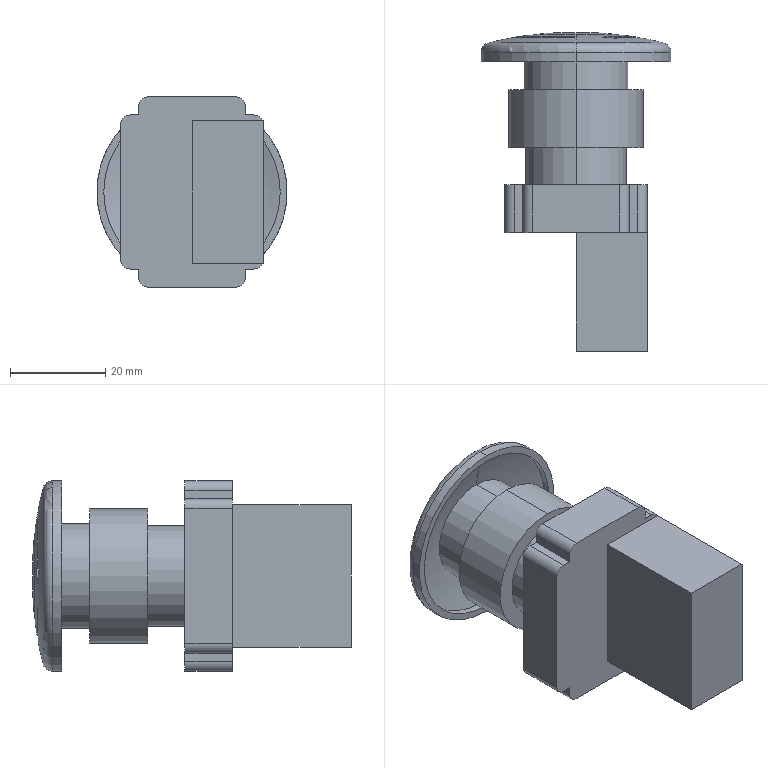Part | SolidWorks | features Cut 3, Fillet 3, Boss 2, Revolution 1 | 3 solids | 85 faces | box 40 x 67.009 x 40 mm | volume 39506 mm3 | plane 43 | cylinder 30 | torus 12 | commonest cylinder face diameters 4 x8 25 x4 27.5 x4 18 x2 19.5 x2 21.2 x2